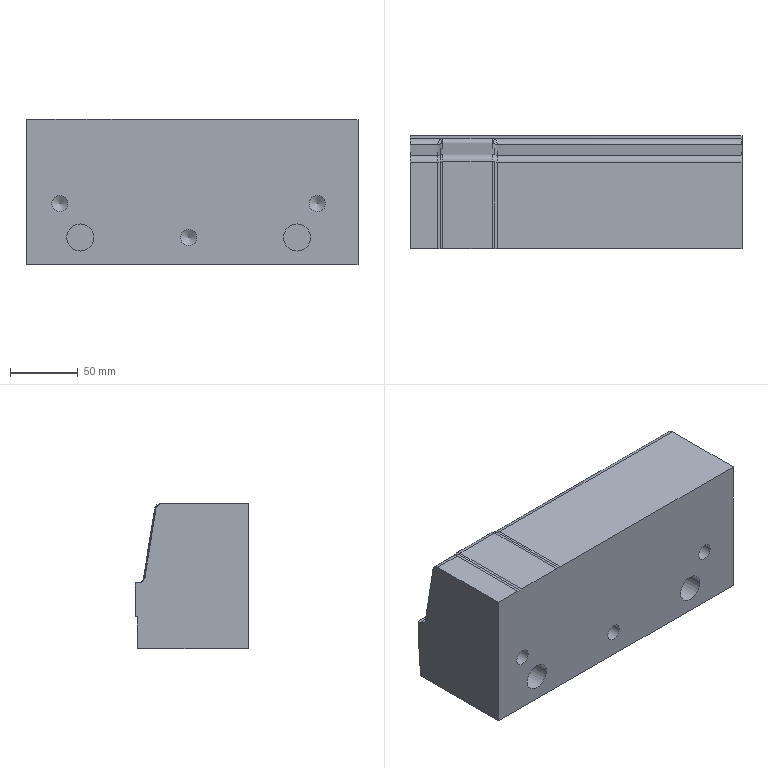Part | NX | features solid 2 | 1 solid | 51 faces | box 245 x 83.473 x 107.229 mm | volume 1994920 mm3 | spline 19 | cylinder 15 | plane 14 | cone 3 | commonest cylinder face diameters 8 x5 10 x5 12 x3 20 x2